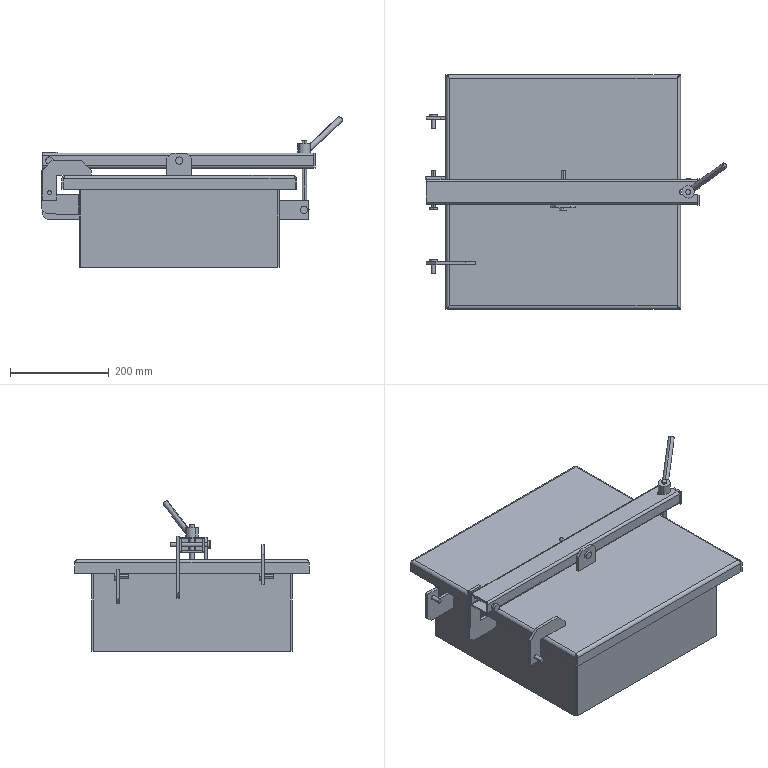Part | SolidWorks | features AEMSimFeature 1, CompositeCurve 1 | 21 solids | 282 faces | box 610.405 x 476 x 304.855 mm | volume 2318365 mm3 | plane 170 | cylinder 86 | spline 24 | cone 2 | commonest cylinder face diameters 9 x20 8 x14 12 x14 15 x10 6 x8 10 x6